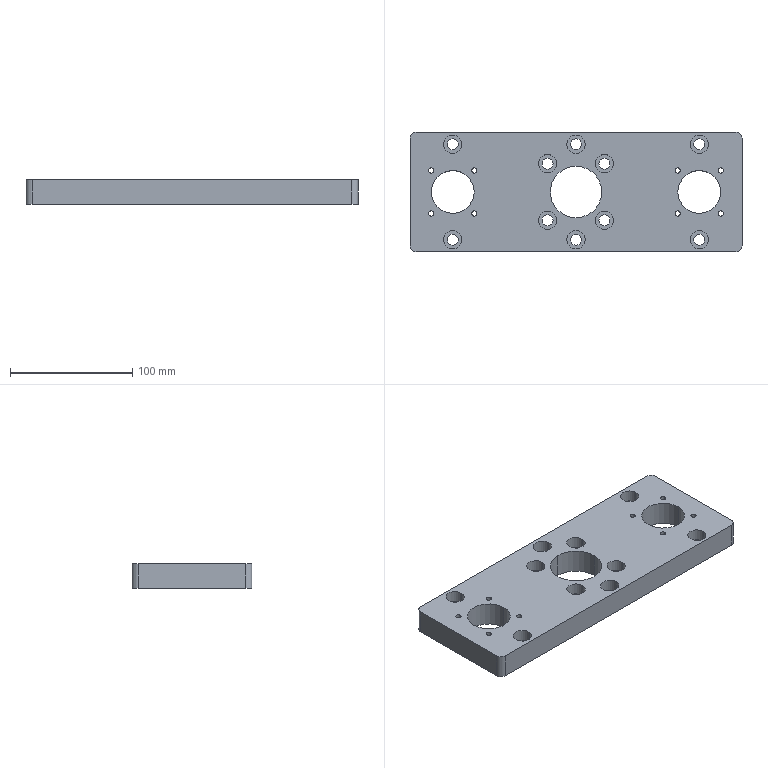Part | 1 solid | 83 faces | box 271.6 x 98 x 20 mm | volume 439441 mm3 | cylinder 67 | plane 16 | commonest cylinder face diameters 9 x20 15 x20 4.2 x16 10 x4 35 x4 42 x3